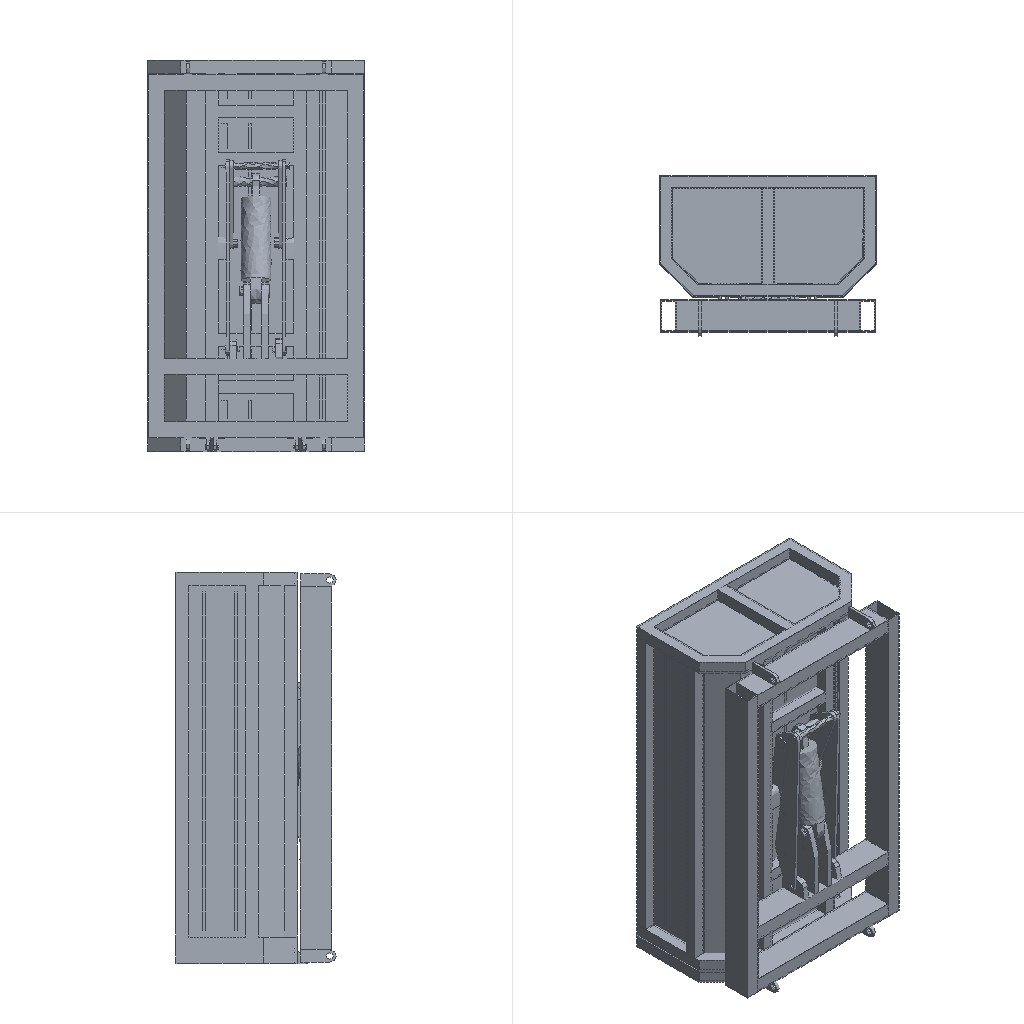Simulation study | ansys workbench
Ansys APDL input file, long lists of numbers shortened:
/batch
/config,noeldb,1     ! force off writing results to database
*get,_wallstrt,active,,time,wall
! ANSYS input file written by Workbench version 2022 R1
! File used for geometry attach:
/title,0-0--____ (A5)
! ****** Begin Custom Load Command Snippet ******
/COM, ACT Extensions:
/COM,     LSDYNA, 2021.1
/COM,
! ****** End   Custom Load Command Snippet ******
*DIM,_wb_ProjectScratch_dir,string,248
_wb_ProjectScratch_dir(1) = ''
*DIM,_wb_SolverFiles_dir,string,248
_wb_SolverFiles_dir(1) = ''
*DIM,_wb_userfiles_dir,string,248
_wb_userfiles_dir(1) = ''
/com,--- Data in consistent MKS units. See Solving Units in the help system for more information.
/units,MKS
/nopr
/wb,file,start              !  signify a WB generated input file
/prep7
! Turn off shape checking because checks already performed inside WB mesher.
! See help system for more information.
SHPP,OFF,,NOWARN
/nolist
etcon,set             ! allow ANSYS to choose best KEYOP's for 180x elements, resets any applicable keyopt to MAPDL defaults
/com,*********** Nodes for the whole assembly ***********
nblock,3,,260693
(1i9,3e20.9e3)
        1    -6.880067124E-02     1.300000000E-02    -8.485000000E-01
! (236993 more lines like these left out)
-1
/com,*********** Nodes for all Remote Points ***********
nblock,3
(1i9,3e20.9e3)
   236995    -1.888006641E-01     1.526826598E-01    -5.740000248E-01
-1
/wb,elem,start            !  set before creation of elements
/com,*********** Elements for Body 1 "__\____-____1" ***********
et,1,186
keyo,1,2,1          ! set full integration on SOLID186
eblock,19,solid,,8004
(19i9)
        1        1        1        1        0        0        0        0       20        0     3161    14707    14708    16320    16321    16180    16179    17757    17756
! (16007 more lines like these left out)
-1
/com,*********** Elements for Body 2 "______3c_____3e_\__________________gb_Mt6728-2002 40__3(1)[6]" ***********
et,2,186
keyo,2,2,1          ! set full integration on SOLID186
eblock,19,solid,,192
(19i9)
        2        2        2        2        0        0        0        0       20        0        1      129      224      416      261      130      189      403      262
! (383 more lines like these left out)
-1
/com,*********** Elements for Body 3 "______3c_____3e_\__________________gb_Mt6728-2002 40__3(1)[4]" ***********
et,3,186
keyo,3,2,1          ! set full integration on SOLID186
eblock,19,solid,,192
(19i9)
        3        3        3        3        0        0        0        0       20        0      193     1515     1527     1681     1707     1516     1550     1682     1708
! (383 more lines like these left out)
-1
/com,*********** Elements for Body 4 "______3c_____3e_\__________________(gb t6728-2002) 40__3(1)[2]" ***********
et,4,187
eblock,19,solid,,9885
(19i9)
        4        4        4        4        0        0        0        0       10        0    11197    60859    60860    62766    61249    65541    65554    65544    65542
! (19769 more lines like these left out)
-1
/com,*********** Elements for Body 5 "_____\____-____1" ***********
et,5,187
eblock,19,solid,,112
(19i9)
        5        5        5        5        0        0        0        0       10        0    94820   226180   226223   226238   226184   226251   226450   226253   226247
! (223 more lines like these left out)
-1
! (32 more sections like these left out)
/wb,elem,end               !  done creating elements
/com,*********** Send User Defined Coordinate System(s) ***********
csys,0
toffst,273.15,  ! Temperature offset from absolute zero
/com,*********** Set Reference Temperature ***********
tref,22.
/wb,mat,start              !  starting to send materials
/com,*********** Send Materials ***********
Temperature = 'TEMP' ! Temperature
MP,DENS,1,7850,	! kg m^-3
MP,ALPX,1,1.2e-05,	! C^-1
MP,C,1,434,	! J kg^-1 C^-1
MP,KXX,1,60.5,	! W m^-1 C^-1
MP,RSVX,1,1.7e-07,	! kg m^3 A^-2 s^-3
MP,EX,1,200000000000,	! Pa
MP,NUXY,1,0.3,
MP,MURX,1,10000,
Temperature = 'TEMP' ! Temperature
MP,DENS,2,7850,	! kg m^-3
MP,ALPX,2,1.2e-05,	! C^-1
MP,C,2,434,	! J kg^-1 C^-1
MP,KXX,2,60.5,	! W m^-1 C^-1
MP,RSVX,2,1.7e-07,	! kg m^3 A^-2 s^-3
MP,EX,2,200000000000,	! Pa
MP,NUXY,2,0.3,
MP,MURX,2,10000,
Temperature = 'TEMP' ! Temperature
MP,DENS,3,7850,	! kg m^-3
MP,ALPX,3,1.2e-05,	! C^-1
MP,C,3,434,	! J kg^-1 C^-1
MP,KXX,3,60.5,	! W m^-1 C^-1
MP,RSVX,3,1.7e-07,	! kg m^3 A^-2 s^-3
MP,EX,3,200000000000,	! Pa
MP,NUXY,3,0.3,
MP,MURX,3,10000,
Temperature = 'TEMP' ! Temperature
MP,DENS,4,7850,	! kg m^-3
MP,ALPX,4,1.2e-05,	! C^-1
MP,C,4,434,	! J kg^-1 C^-1
MP,KXX,4,60.5,	! W m^-1 C^-1
MP,RSVX,4,1.7e-07,	! kg m^3 A^-2 s^-3
MP,EX,4,200000000000,	! Pa
MP,NUXY,4,0.3,
MP,MURX,4,10000,
Temperature = 'TEMP' ! Temperature
MP,DENS,5,7850,	! kg m^-3
MP,ALPX,5,1.2e-05,	! C^-1
MP,C,5,434,	! J kg^-1 C^-1
MP,KXX,5,60.5,	! W m^-1 C^-1
MP,RSVX,5,1.7e-07,	! kg m^3 A^-2 s^-3
MP,EX,5,200000000000,	! Pa
MP,NUXY,5,0.3,
MP,MURX,5,10000,
Temperature = 'TEMP' ! Temperature
MP,DENS,6,7850,	! kg m^-3
MP,ALPX,6,1.2e-05,	! C^-1
MP,C,6,434,	! J kg^-1 C^-1
MP,KXX,6,60.5,	! W m^-1 C^-1
MP,RSVX,6,1.7e-07,	! kg m^3 A^-2 s^-3
MP,EX,6,200000000000,	! Pa
MP,NUXY,6,0.3,
MP,MURX,6,10000,
Temperature = 'TEMP' ! Temperature
MP,DENS,7,7850,	! kg m^-3
MP,ALPX,7,1.2e-05,	! C^-1
MP,C,7,434,	! J kg^-1 C^-1
MP,KXX,7,60.5,	! W m^-1 C^-1
MP,RSVX,7,1.7e-07,	! kg m^3 A^-2 s^-3
MP,EX,7,200000000000,	! Pa
MP,NUXY,7,0.3,
MP,MURX,7,10000,
Temperature = 'TEMP' ! Temperature
MP,DENS,8,7850,	! kg m^-3
MP,ALPX,8,1.2e-05,	! C^-1
MP,C,8,434,	! J kg^-1 C^-1
MP,KXX,8,60.5,	! W m^-1 C^-1
MP,RSVX,8,1.7e-07,	! kg m^3 A^-2 s^-3
MP,EX,8,200000000000,	! Pa
MP,NUXY,8,0.3,
MP,MURX,8,10000,
Temperature = 'TEMP' ! Temperature
MP,DENS,9,7850,	! kg m^-3
MP,ALPX,9,1.2e-05,	! C^-1
MP,C,9,434,	! J kg^-1 C^-1
MP,KXX,9,60.5,	! W m^-1 C^-1
MP,RSVX,9,1.7e-07,	! kg m^3 A^-2 s^-3
MP,EX,9,200000000000,	! Pa
! (254 more lines like these left out)
/wb,mat,end                !  done sending materials
!************************* Model Summary ********************
!__\____-____1,	结构钢,	matid,	1
!______3c_____3e_\__________________gb_Mt6728-2002 40__3(1)[6],	结构钢,	matid,	2
!______3c_____3e_\__________________gb_Mt6728-2002 40__3(1)[4],	结构钢,	matid,	3
! (36 more lines like these left out)
*get,_xmin,node,,mnloc,x
*get,_ymin,node,,mnloc,y
*get,_zmin,node,,mnloc,z
*get,_xmax,node,,mxloc,x
*get,_ymax,node,,mxloc,y
*get,_zmax,node,,mxloc,z
_ASMDIAG=(_xmax-_xmin)*(_xmax-_xmin)+(_ymax-_ymin)*(_ymax-_ymin)+(_zmax-_zmin)*(_zmax-_zmin)
_ASMDIAG=SQRT(_ASMDIAG)
/wb,contact,start          !  starting to send contact
/com,*********** Create Contact "接触区域" ***********
/com,            Real Constant Set For Above Contact Is 39 & 38
*set,tid,39
*set,cid,38
r,tid
r,cid
et,tid,170
et,cid,174
eblock,10,,,87
(15i9)
   173247       39       39       39        0    11794    11795    11738    11737    32820    32597    32592    32593
! (86 more lines like these left out)
-1
eblock,10,,,87
(15i9)
   173334       38       38       38        0    11794    11795    11738    11737    32820    32597    32592    32593
! (86 more lines like these left out)
-1
eblock,10,,,48
(15i9)
   173421       38       39       38        0       66       33       70       69      499      500      614      608
! (47 more lines like these left out)
-1
eblock,10,,,48
(15i9)
   173469       39       38       39        0       66       33       70       69      499      500      614      608
! (47 more lines like these left out)
-1
keyo,cid,8,2               ! auto create asymmetric contact (from Program Controlled setting)
keyo,cid,10,0              ! adjust contact stiffness each NR iteration (from Program Controlled setting)
keyo,cid,12,5              ! bonded always
keyo,cid,2,2               ! MPC contact.  Valid only for bonded or no separation.  Requires nodal detection
keyo,cid,4,2               ! on nodal point - normal to target surface (from Program Controlled setting)
keyo,cid,9,1               ! ignore initial gaps/penetration
keyo,cid,7,0               ! No Prediction
rmod,tid,3,10.      ! FKN
rmod,tid,5,0.       ! ICONT
rmod,tid,6,-3.e-003 ! PINB
rmod,tid,10,0.      ! CNOF
rmod,tid,12,0.      ! FKT
rmod,tid,36,140     ! WB DSID
rmod,cid,3,10.      ! FKN
rmod,cid,5,0.       ! ICONT
rmod,cid,6,-3.e-003 ! PINB
rmod,cid,10,0.      ! CNOF
rmod,cid,12,0.      ! FKT
rmod,cid,36,140     ! WB DSID
/com,*********** Create Contact "接触区域 2" ***********
/com,            Real Constant Set For Above Contact Is 41 & 40
*set,tid,41
*set,cid,40
r,tid
r,cid
et,tid,170
et,cid,174
eblock,10,,,116
(15i9)
   173517       41       41       41        0    11786    11787    11730    11729    32788    32565    32560    32561
! (115 more lines like these left out)
-1
eblock,10,,,116
(15i9)
   173633       40       40       40        0    11786    11787    11730    11729    32788    32565    32560    32561
! (115 more lines like these left out)
-1
eblock,10,,,48
(15i9)
   173749       40       41       40        0     1455     1457     1493     1456     1919     1923     1920     1918
! (47 more lines like these left out)
-1
eblock,10,,,48
(15i9)
   173797       41       40       41        0     1455     1457     1493     1456     1919     1923     1920     1918
! (47 more lines like these left out)
-1
keyo,cid,8,2               ! auto create asymmetric contact (from Program Controlled setting)
keyo,cid,10,0              ! adjust contact stiffness each NR iteration (from Program Controlled setting)
keyo,cid,12,5              ! bonded always
keyo,cid,2,2               ! MPC contact.  Valid only for bonded or no separation.  Requires nodal detection
keyo,cid,4,2               ! on nodal point - normal to target surface (from Program Controlled setting)
keyo,cid,9,1               ! ignore initial gaps/penetration
keyo,cid,7,0               ! No Prediction
rmod,tid,3,10.      ! FKN
rmod,tid,5,0.       ! ICONT
rmod,tid,6,-3.e-003 ! PINB
rmod,tid,10,0.      ! CNOF
rmod,tid,12,0.      ! FKT
rmod,tid,36,143     ! WB DSID
rmod,cid,3,10.      ! FKN
rmod,cid,5,0.       ! ICONT
rmod,cid,6,-3.e-003 ! PINB
rmod,cid,10,0.      ! CNOF
rmod,cid,12,0.      ! FKT
rmod,cid,36,143     ! WB DSID
/com,*********** Create Contact "接触区域 3" ***********
/com,            Real Constant Set For Above Contact Is 43 & 42
*set,tid,43
*set,cid,42
r,tid
r,cid
et,tid,170
et,cid,174
eblock,10,,,138
(15i9)
   173845       43       43       43        0    16178    17757    16179    16179    46419    46421    16179    46418
! (137 more lines like these left out)
-1
eblock,10,,,138
(15i9)
   173983       42       42       42        0    16178    17757    16179    16179    46419    46421    16179    46418
! (137 more lines like these left out)
-1
eblock,10,,,135
(15i9)
   174121       42       43       42        0    62662    62758    62759    62759    76459    77401    62759    76460
! (134 more lines like these left out)
-1
eblock,10,,,135
(15i9)
   174256       43       42       43        0    62662    62758    62759    62759    76459    77401    62759    76460
! (134 more lines like these left out)
-1
keyo,cid,8,2               ! auto create asymmetric contact (from Program Controlled setting)
keyo,cid,10,0              ! adjust contact stiffness each NR iteration (from Program Controlled setting)
keyo,cid,12,5              ! bonded always
keyo,cid,2,2               ! MPC contact.  Valid only for bonded or no separation.  Requires nodal detection
keyo,cid,4,2               ! on nodal point - normal to target surface (from Program Controlled setting)
keyo,cid,9,1               ! ignore initial gaps/penetration
keyo,cid,7,0               ! No Prediction
rmod,tid,3,10.      ! FKN
rmod,tid,5,0.       ! ICONT
rmod,tid,6,-3.e-003 ! PINB
rmod,tid,10,0.      ! CNOF
rmod,tid,12,0.      ! FKT
rmod,tid,36,146     ! WB DSID
rmod,cid,3,10.      ! FKN
rmod,cid,5,0.       ! ICONT
rmod,cid,6,-3.e-003 ! PINB
rmod,cid,10,0.      ! CNOF
rmod,cid,12,0.      ! FKT
rmod,cid,36,146     ! WB DSID
/com,*********** Create Contact "接触区域 8" ***********
/com,            Real Constant Set For Above Contact Is 45 & 44
*set,tid,45
*set,cid,44
r,tid
r,cid
et,tid,170
et,cid,174
eblock,10,,,2963
(15i9)
   174391       45       45       45        0    10487     8948     8891     8890    24139    24025    24022    24023
! (2962 more lines like these left out)
-1
eblock,10,,,2963
(15i9)
   177354       44       44       44        0    10487     8948     8891     8890    24139    24025    24022    24023
! (2962 more lines like these left out)
-1
eblock,10,,,3021
(15i9)
   180317       44       45       44        0   140312   149120   144739   144739   167185   199225   144739   167183
! (3020 more lines like these left out)
-1
eblock,10,,,3021
(15i9)
   183338       45       44       45        0   140312   149120   144739   144739   167185   199225   144739   167183
! (3020 more lines like these left out)
-1
keyo,cid,8,2               ! auto create asymmetric contact (from Program Controlled setting)
keyo,cid,10,0              ! adjust contact stiffness each NR iteration (from Program Controlled setting)
keyo,cid,12,5              ! bonded always
keyo,cid,2,2               ! MPC contact.  Valid only for bonded or no separation.  Requires nodal detection
keyo,cid,4,2               ! on nodal point - normal to target surface (from Program Controlled setting)
keyo,cid,9,1               ! ignore initial gaps/penetration
keyo,cid,7,0               ! No Prediction
rmod,tid,3,10.      ! FKN
rmod,tid,5,0.       ! ICONT
rmod,tid,6,-3.e-003 ! PINB
rmod,tid,10,0.      ! CNOF
rmod,tid,12,0.      ! FKT
rmod,tid,36,161     ! WB DSID
rmod,cid,3,10.      ! FKN
rmod,cid,5,0.       ! ICONT
rmod,cid,6,-3.e-003 ! PINB
rmod,cid,10,0.      ! CNOF
rmod,cid,12,0.      ! FKT
rmod,cid,36,161     ! WB DSID
/com,*********** Create Contact "接触区域 9" ***********
/com,            Real Constant Set For Above Contact Is 47 & 46
*set,tid,47
*set,cid,46
r,tid
r,cid
et,tid,170
et,cid,174
eblock,10,,,32
(15i9)
   186359       47       47       47        0       24       17        3       12      466      425      424      452
! (31 more lines like these left out)
-1
eblock,10,,,32
(15i9)
   186391       46       46       46        0       24       17        3       12      466      425      424      452
! (31 more lines like these left out)
-1
eblock,10,,,44
(15i9)
   186423       46       47       46        0   139696   152203   144107   144107   162593   196407   144107   162590
! (43 more lines like these left out)
-1
eblock,10,,,44
(15i9)
   186467       47       46       47        0   139696   152203   144107   144107   162593   196407   144107   162590
! (43 more lines like these left out)
-1
keyo,cid,8,2               ! auto create asymmetric contact (from Program Controlled setting)
keyo,cid,10,0              ! adjust contact stiffness each NR iteration (from Program Controlled setting)
keyo,cid,12,5              ! bonded always
keyo,cid,2,2               ! MPC contact.  Valid only for bonded or no separation.  Requires nodal detection
keyo,cid,4,2               ! on nodal point - normal to target surface (from Program Controlled setting)
keyo,cid,9,1               ! ignore initial gaps/penetration
keyo,cid,7,0               ! No Prediction
rmod,tid,3,10.      ! FKN
rmod,tid,5,0.       ! ICONT
rmod,tid,6,-3.e-003 ! PINB
rmod,tid,10,0.      ! CNOF
rmod,tid,12,0.      ! FKT
rmod,tid,36,164     ! WB DSID
rmod,cid,3,10.      ! FKN
rmod,cid,5,0.       ! ICONT
rmod,cid,6,-3.e-003 ! PINB
rmod,cid,10,0.      ! CNOF
rmod,cid,12,0.      ! FKT
rmod,cid,36,164     ! WB DSID
! (43 more sections like these left out)
/wb,contact,end            !  done creating contacts
/golist
/wb,load,start             !  starting to send loads
/com,*********** Fixed Supports ***********
CMBLOCK,_FIXEDSU,NODE,      160
(8i10)
     60339     60340     60341     60342     60343     60344     60345     60346
! (19 more lines like these left out)
cmsel,s,_FIXEDSU
d,all,all
nsel,all
/com,*********** Create Remote Point "内部远程点" ***********
! -------- Remote Point Used by "点质量" --------
*set,tid,135
*set,cid,134
et,cid,174
et,tid,170
keyo,tid,2,1               ! Don't fix the pilot node
keyo,tid,4,000111
keyo,cid,12,5              ! Bonded Contact
keyo,cid,4,3               ! Coupled CPINTF style load
keyo,cid,2,2               ! MPC style contact
eblock,10,,,6960
(15i9)
   192867      134      134      134        0    21013    18518    21011    21012    51061    51060    56002    56003
! (6959 more lines like these left out)
-1
*set,_npilot,236995
_npilot352=_npilot
type,tid
mat ,cid
real,cid
tshape,pilo
en,199827,_npilot
tshape
/com,*********** Define Force Using Surface Effect Elements ***********
local,12,0,0.,0.,0.,0.,0.,0.
csys,0
et,136,154
eblock,10,,,20
(15i9)
   199828      136      136      136       12     2869     2877     2871     2871     3146     3153     2871     3145
! (19 more lines like these left out)
-1
esel,s,type,,136
keyop,136,2,1                ! Apply load in local coordinate system
keyop,136,7,1                ! Use original area so load is constant in large deformation
esel,all
/com,*********** Define Force Using Surface Effect Elements ***********
local,13,0,0.,0.,0.,0.,0.,0.
csys,0
et,137,154
eblock,10,,,22
(15i9)
   199848      137      137      137       13     3855     3857     4155     4155     4408     4424     4155     4412
! (21 more lines like these left out)
-1
esel,s,type,,137
keyop,137,2,1                ! Apply load in local coordinate system
keyop,137,7,1                ! Use original area so load is constant in large deformation
esel,all
/com,*********** Construct Remote Mass Using Remote Attachment ***********
*set,_tid,138
et,_tid,21           ! MASS21 element
type,_tid
mat ,_tid
real,_tid
keyo,_tid,3,2        ! 3d mass without rotary inertia
r,_tid,600.
en,199870,236995
/gst,on,on
fini
*get,_numnode,node,0,count
*get,_numelem,elem,0,count
*get, _MAXELEMNUM, elem, 0, NUM, MAX
*get, _MAXNODENUM, node, 0, NUM, MAX
*get, _MAXELEMTYPE, etyp, 0, NUM, MAX
*get, _MAXREALCONST, real, 0, NUM, MAX
/go
/wb,load,end               !  done creating loads
/com,--- Number of total nodes = %_numnode%
/com,--- Number of contact elements = 26622
/com,--- Number of spring elements = 0
/com,--- Number of bearing elements = 0
/com,--- Number of solid elements = 97917
/com,--- Number of condensed parts = 0
/com,--- Number of total elements = %_numelem%
*get,_wallbsol,active,,time,wall
/com,****************************************************************************
/com,*************************    SOLUTION       ********************************
/com,****************************************************************************
/solu
antype,0                   ! static analysis
neqit,1,force              ! Force 1 eq iteration since only nonlinearity is bonded/no sep contact
pred,off
_thickRatio=0.135   ! Ratio of thick parts in the model
eqsl,sparse,,,,,1
cntr,print,1               ! print out contact info and also make no initial contact an error
dmpoption,emat,no             ! Don't combine emat file for DANSYS
dmpoption,esav,no             ! Don't combine esav file for DANSYS
nldiag,cont,iter           ! print out contact info each equilibrium iteration
rescontrol,,none                 ! Do not keep any restart files
/com,****************************************************
/com,******************* SOLVE FOR LS 1 OF 1 ****************
esel,s,type,,136
nsle
sfe,all,1,pres,1,0.
sfe,all,2,pres,1,1620761.678
sfe,all,3,pres,1,10411212.772
esel,s,type,,137
nsle
sfe,all,1,pres,1,6.74034122059795e-009
sfe,all,2,pres,1,-1049300.184
sfe,all,3,pres,1,-6740341.67
nsel,all
esel,all
acel,0.,9.807,0.
/nopr
/gopr
nsub,1,1,1
time,1.
outres,erase
outres,all,none
outres,nsol,all,
outres,rsol,all
outres,eangl,all
outres,etmp,all
outres,veng,all
outres,strs,all,
outres,epel,all,
outres,eppl,all,
outres,cont,all,
! *********** WB SOLVE COMMAND ***********
! check interactive state
*get,ANSINTER_,active,,int
*if,ANSINTER_,ne,0,then
/eof
*endif
solve
/com *************** Write FE CONNECTORS *********
CEWRITE,file,ce,,INTE
/com,****************************************************
/com,*************** FINISHED SOLVE FOR LS 1 *************
*get,_wallasol,active,,time,wall
/nopr
*get,_numnode,node,0,count
*get,_numelem,elem,0,count
*get, _MAXELEMNUM, elem, 0, NUM, MAX
*get, _MAXNODENUM, node, 0, NUM, MAX,,,INTERNAL
*get, _MAXELEMTYPE, etyp, 0, NUM, MAX
*get, _MAXREALCONST, real, 0, NUM, MAX
/gopr
/post1
xmlo,ENCODING,ISO-8859-1
xmlo,parm
/xml,parm,xml
fini
/gopr
*get,_walldone,active,,time,wall
_preptime=(_wallbsol-_wallstrt)*3600
_solvtime=(_wallasol-_wallbsol)*3600
_posttime=(_walldone-_wallasol)*3600
_totaltim=(_walldone-_wallstrt)*3600
*get,_dlbratio,active,0,solu,dlbr
*get,_combtime,active,0,solu,comb
*get,_ssmode,active,0,solu,ssmm
*get,_ndofs,active,0,solu,ndof
*get,_sol_end_time,active,0,set,time
*if,_sol_end_time,eq,1.,then
/fclean				!clean distributed files
*endif
/com,--- Total number of nodes = %_numnode%
/com,--- Total number of elements = %_numelem%
/com,--- Element load balance ratio = %_dlbratio%
/com,--- Time to combine distributed files = %_combtime%
/com,--- Sparse memory mode = %_ssmode%
/com,--- Number of DOF = %_ndofs%
/wb,file,end               ! done with WB generated input